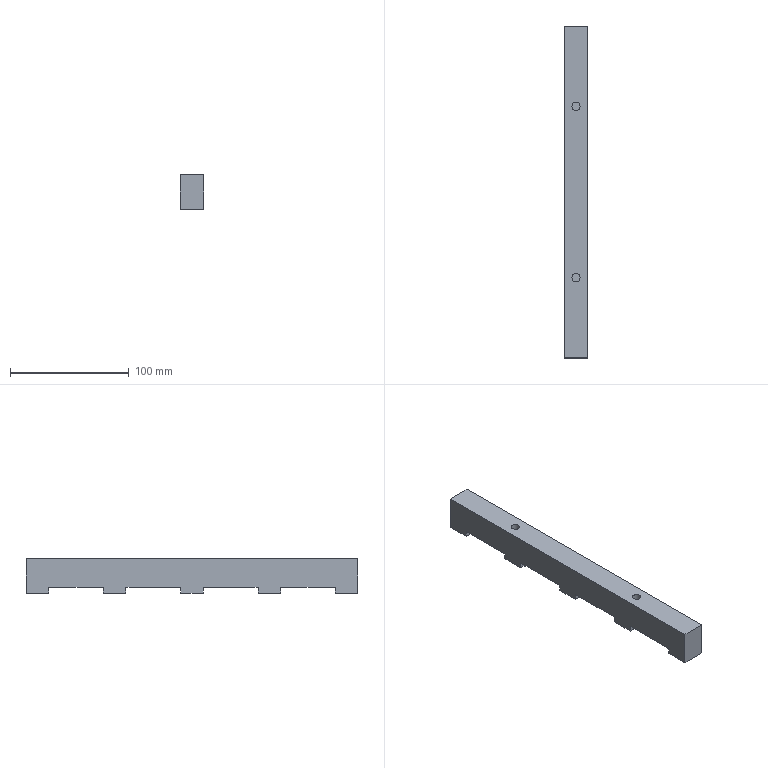Part | NX | 1 solid | 26 faces | box 20 x 279 x 29 mm | volume 142481 mm3 | plane 24 | cylinder 2 | commonest cylinder face diameters 6.88 x2
STEP:
#1=CARTESIAN_POINT('',(75.884,204.443,-119.05));
#2=VERTEX_POINT('',#1);
#3=CARTESIAN_POINT('',(72.444,204.443,-119.05));
#4=DIRECTION('',(0.,0.,-1.));
#5=DIRECTION('',(1.,0.,0.));
#6=AXIS2_PLACEMENT_3D('',#3,#4,#5);
#7=CIRCLE('',#6,3.44);
#8=EDGE_CURVE('',#2,#2,#7,.T.);
#9=ORIENTED_EDGE('',*,*,#8,.T.);
#10=EDGE_LOOP('',(#9));
#11=FACE_BOUND('',#10,.T.);
#12=CARTESIAN_POINT('',(75.884,204.443,-106.3));
#13=VERTEX_POINT('',#12);
#14=CARTESIAN_POINT('',(72.444,204.443,-106.3));
#15=DIRECTION('',(0.,0.,1.));
#16=DIRECTION('',(1.,0.,0.));
#17=AXIS2_PLACEMENT_3D('',#14,#15,#16);
#18=CIRCLE('',#17,3.44);
#19=EDGE_CURVE('',#13,#13,#18,.T.);
#20=ORIENTED_EDGE('',*,*,#19,.T.);
#21=EDGE_LOOP('',(#20));
#22=FACE_BOUND('',#21,.T.);
#23=CARTESIAN_POINT('',(72.444,204.443,-99.05));
#24=DIRECTION('',(0.,0.,-1.));
#25=DIRECTION('',(1.,0.,0.));
#26=AXIS2_PLACEMENT_3D('',#23,#24,#25);
#27=CYLINDRICAL_SURFACE('',#26,3.44);
#28=ADVANCED_FACE('',(#11,#22),#27,.F.);
#29=ORIENTED_EDGE('',*,*,#8,.F.);
#30=EDGE_LOOP('',(#29));
#31=FACE_BOUND('',#30,.T.);
#32=CARTESIAN_POINT('',(72.444,204.443,-119.05));
#33=DIRECTION('',(0.,0.,-1.));
#34=DIRECTION('',(-1.,0.,0.));
#35=AXIS2_PLACEMENT_3D('',#32,#33,#34);
#36=PLANE('',#35);
#37=ADVANCED_FACE('',(#31),#36,.F.);
#38=CARTESIAN_POINT('',(75.884,348.443,-118.8));
#39=VERTEX_POINT('',#38);
#40=CARTESIAN_POINT('',(72.444,348.443,-118.8));
#41=DIRECTION('',(0.,0.,-1.));
#42=DIRECTION('',(1.,0.,0.));
#43=AXIS2_PLACEMENT_3D('',#40,#41,#42);
#44=CIRCLE('',#43,3.44);
#45=EDGE_CURVE('',#39,#39,#44,.T.);
#46=ORIENTED_EDGE('',*,*,#45,.T.);
#47=EDGE_LOOP('',(#46));
#48=FACE_BOUND('',#47,.T.);
#49=CARTESIAN_POINT('',(75.884,348.443,-106.3));
#50=VERTEX_POINT('',#49);
#51=CARTESIAN_POINT('',(72.444,348.443,-106.3));
#52=DIRECTION('',(0.,0.,1.));
#53=DIRECTION('',(1.,0.,0.));
#54=AXIS2_PLACEMENT_3D('',#51,#52,#53);
#55=CIRCLE('',#54,3.44);
#56=EDGE_CURVE('',#50,#50,#55,.T.);
#57=ORIENTED_EDGE('',*,*,#56,.T.);
#58=EDGE_LOOP('',(#57));
#59=FACE_BOUND('',#58,.T.);
#60=CARTESIAN_POINT('',(72.444,348.443,-98.8));
#61=DIRECTION('',(0.,0.,-1.));
#62=DIRECTION('',(1.,0.,0.));
#63=AXIS2_PLACEMENT_3D('',#60,#61,#62);
#64=CYLINDRICAL_SURFACE('',#63,3.44);
#65=ADVANCED_FACE('',(#48,#59),#64,.F.);
#66=ORIENTED_EDGE('',*,*,#45,.F.);
#67=EDGE_LOOP('',(#66));
#68=FACE_BOUND('',#67,.T.);
#69=CARTESIAN_POINT('',(72.444,348.443,-118.8));
#70=DIRECTION('',(0.,0.,-1.));
#71=DIRECTION('',(-1.,0.,0.));
#72=AXIS2_PLACEMENT_3D('',#69,#70,#71);
#73=PLANE('',#72);
#74=ADVANCED_FACE('',(#68),#73,.F.);
#75=CARTESIAN_POINT('',(82.444,155.943,-130.3));
#76=VERTEX_POINT('',#75);
#77=CARTESIAN_POINT('',(82.444,155.943,-135.3));
#78=VERTEX_POINT('',#77);
#79=CARTESIAN_POINT('',(82.444,155.943,-130.75));
#80=DIRECTION('',(0.,0.,-1.));
#81=VECTOR('',#80,1000.);
#82=LINE('',#79,#81);
#83=EDGE_CURVE('',#76,#78,#82,.T.);
#84=ORIENTED_EDGE('',*,*,#83,.T.);
#85=CARTESIAN_POINT('',(62.444,155.943,-135.3));
#86=VERTEX_POINT('',#85);
#87=CARTESIAN_POINT('',(72.444,155.943,-135.3));
#88=DIRECTION('',(-1.,0.,0.));
#89=VECTOR('',#88,1000.);
#90=LINE('',#87,#89);
#91=EDGE_CURVE('',#78,#86,#90,.T.);
#92=ORIENTED_EDGE('',*,*,#91,.T.);
#93=CARTESIAN_POINT('',(62.444,155.943,-130.3));
#94=VERTEX_POINT('',#93);
#95=CARTESIAN_POINT('',(62.444,155.943,-139.8));
#96=DIRECTION('',(0.,0.,-1.));
#97=VECTOR('',#96,1000.);
#98=LINE('',#95,#97);
#99=EDGE_CURVE('',#94,#86,#98,.T.);
#100=ORIENTED_EDGE('',*,*,#99,.F.);
#101=CARTESIAN_POINT('',(113.544,155.943,-130.3));
#102=DIRECTION('',(1.,0.,0.));
#103=VECTOR('',#102,1000.);
#104=LINE('',#101,#103);
#105=EDGE_CURVE('',#94,#76,#104,.T.);
#106=ORIENTED_EDGE('',*,*,#105,.T.);
#107=EDGE_LOOP('',(#84,#92,#100,#106));
#108=FACE_BOUND('',#107,.T.);
#109=CARTESIAN_POINT('',(113.544,155.943,-130.75));
#110=DIRECTION('',(0.,1.,0.));
#111=DIRECTION('',(-1.,0.,0.));
#112=AXIS2_PLACEMENT_3D('',#109,#110,#111);
#113=PLANE('',#112);
#114=ADVANCED_FACE('',(#108),#113,.T.);
#115=CARTESIAN_POINT('',(62.444,201.943,-135.3));
#116=VERTEX_POINT('',#115);
#117=CARTESIAN_POINT('',(62.444,201.943,-130.3));
#118=VERTEX_POINT('',#117);
#119=CARTESIAN_POINT('',(62.444,201.943,-139.8));
#120=DIRECTION('',(0.,0.,1.));
#121=VECTOR('',#120,1000.);
#122=LINE('',#119,#121);
#123=EDGE_CURVE('',#116,#118,#122,.T.);
#124=ORIENTED_EDGE('',*,*,#123,.F.);
#125=CARTESIAN_POINT('',(82.444,201.943,-135.3));
#126=VERTEX_POINT('',#125);
#127=CARTESIAN_POINT('',(72.444,201.943,-135.3));
#128=DIRECTION('',(1.,0.,0.));
#129=VECTOR('',#128,1000.);
#130=LINE('',#127,#129);
#131=EDGE_CURVE('',#116,#126,#130,.T.);
#132=ORIENTED_EDGE('',*,*,#131,.T.);
#133=CARTESIAN_POINT('',(82.444,201.943,-130.3));
#134=VERTEX_POINT('',#133);
#135=CARTESIAN_POINT('',(82.444,201.943,-139.85));
#136=DIRECTION('',(0.,0.,1.));
#137=VECTOR('',#136,1000.);
#138=LINE('',#135,#137);
#139=EDGE_CURVE('',#126,#134,#138,.T.);
#140=ORIENTED_EDGE('',*,*,#139,.T.);
#141=CARTESIAN_POINT('',(72.444,201.943,-130.3));
#142=DIRECTION('',(-1.,0.,0.));
#143=VECTOR('',#142,1000.);
#144=LINE('',#141,#143);
#145=EDGE_CURVE('',#134,#118,#144,.T.);
#146=ORIENTED_EDGE('',*,*,#145,.T.);
#147=EDGE_LOOP('',(#124,#132,#140,#146));
#148=FACE_BOUND('',#147,.T.);
#149=CARTESIAN_POINT('',(113.544,201.943,-139.85));
#150=DIRECTION('',(0.,-1.,0.));
#151=DIRECTION('',(1.,0.,0.));
#152=AXIS2_PLACEMENT_3D('',#149,#150,#151);
#153=PLANE('',#152);
#154=ADVANCED_FACE('',(#148),#153,.T.);
#155=CARTESIAN_POINT('',(82.444,220.943,-130.3));
#156=VERTEX_POINT('',#155);
#157=CARTESIAN_POINT('',(82.444,220.943,-135.3));
#158=VERTEX_POINT('',#157);
#159=CARTESIAN_POINT('',(82.444,220.943,-130.75));
#160=DIRECTION('',(0.,0.,-1.));
#161=VECTOR('',#160,1000.);
#162=LINE('',#159,#161);
#163=EDGE_CURVE('',#156,#158,#162,.T.);
#164=ORIENTED_EDGE('',*,*,#163,.T.);
#165=CARTESIAN_POINT('',(62.444,220.943,-135.3));
#166=VERTEX_POINT('',#165);
#167=CARTESIAN_POINT('',(72.444,220.943,-135.3));
#168=DIRECTION('',(-1.,0.,0.));
#169=VECTOR('',#168,1000.);
#170=LINE('',#167,#169);
#171=EDGE_CURVE('',#158,#166,#170,.T.);
#172=ORIENTED_EDGE('',*,*,#171,.T.);
#173=CARTESIAN_POINT('',(62.444,220.943,-130.3));
#174=VERTEX_POINT('',#173);
#175=CARTESIAN_POINT('',(62.444,220.943,-139.8));
#176=DIRECTION('',(0.,0.,-1.));
#177=VECTOR('',#176,1000.);
#178=LINE('',#175,#177);
#179=EDGE_CURVE('',#174,#166,#178,.T.);
#180=ORIENTED_EDGE('',*,*,#179,.F.);
#181=CARTESIAN_POINT('',(113.544,220.943,-130.3));
#182=DIRECTION('',(1.,0.,0.));
#183=VECTOR('',#182,1000.);
#184=LINE('',#181,#183);
#185=EDGE_CURVE('',#174,#156,#184,.T.);
#186=ORIENTED_EDGE('',*,*,#185,.T.);
#187=EDGE_LOOP('',(#164,#172,#180,#186));
#188=FACE_BOUND('',#187,.T.);
#189=CARTESIAN_POINT('',(113.544,220.943,-130.75));
#190=DIRECTION('',(0.,1.,0.));
#191=DIRECTION('',(-1.,0.,0.));
#192=AXIS2_PLACEMENT_3D('',#189,#190,#191);
#193=PLANE('',#192);
#194=ADVANCED_FACE('',(#188),#193,.T.);
#195=CARTESIAN_POINT('',(62.444,266.943,-135.3));
#196=VERTEX_POINT('',#195);
#197=CARTESIAN_POINT('',(62.444,266.943,-130.3));
#198=VERTEX_POINT('',#197);
#199=CARTESIAN_POINT('',(62.444,266.943,-139.8));
#200=DIRECTION('',(0.,0.,1.));
#201=VECTOR('',#200,1000.);
#202=LINE('',#199,#201);
#203=EDGE_CURVE('',#196,#198,#202,.T.);
#204=ORIENTED_EDGE('',*,*,#203,.F.);
#205=CARTESIAN_POINT('',(82.444,266.943,-135.3));
#206=VERTEX_POINT('',#205);
#207=CARTESIAN_POINT('',(72.444,266.943,-135.3));
#208=DIRECTION('',(1.,0.,0.));
#209=VECTOR('',#208,1000.);
#210=LINE('',#207,#209);
#211=EDGE_CURVE('',#196,#206,#210,.T.);
#212=ORIENTED_EDGE('',*,*,#211,.T.);
#213=CARTESIAN_POINT('',(82.444,266.943,-130.3));
#214=VERTEX_POINT('',#213);
#215=CARTESIAN_POINT('',(82.444,266.943,-139.85));
#216=DIRECTION('',(0.,0.,1.));
#217=VECTOR('',#216,1000.);
#218=LINE('',#215,#217);
#219=EDGE_CURVE('',#206,#214,#218,.T.);
#220=ORIENTED_EDGE('',*,*,#219,.T.);
#221=CARTESIAN_POINT('',(113.544,266.943,-130.3));
#222=DIRECTION('',(-1.,0.,0.));
#223=VECTOR('',#222,1000.);
#224=LINE('',#221,#223);
#225=EDGE_CURVE('',#214,#198,#224,.T.);
#226=ORIENTED_EDGE('',*,*,#225,.T.);
#227=EDGE_LOOP('',(#204,#212,#220,#226));
#228=FACE_BOUND('',#227,.T.);
#229=CARTESIAN_POINT('',(113.544,266.943,-139.85));
#230=DIRECTION('',(0.,-1.,0.));
#231=DIRECTION('',(1.,0.,0.));
#232=AXIS2_PLACEMENT_3D('',#229,#230,#231);
#233=PLANE('',#232);
#234=ADVANCED_FACE('',(#228),#233,.T.);
#235=CARTESIAN_POINT('',(82.444,285.943,-130.3));
#236=VERTEX_POINT('',#235);
#237=CARTESIAN_POINT('',(82.444,285.943,-135.3));
#238=VERTEX_POINT('',#237);
#239=CARTESIAN_POINT('',(82.444,285.943,-130.75));
#240=DIRECTION('',(0.,0.,-1.));
#241=VECTOR('',#240,1000.);
#242=LINE('',#239,#241);
#243=EDGE_CURVE('',#236,#238,#242,.T.);
#244=ORIENTED_EDGE('',*,*,#243,.T.);
#245=CARTESIAN_POINT('',(62.444,285.943,-135.3));
#246=VERTEX_POINT('',#245);
#247=CARTESIAN_POINT('',(72.444,285.943,-135.3));
#248=DIRECTION('',(-1.,0.,0.));
#249=VECTOR('',#248,1000.);
#250=LINE('',#247,#249);
#251=EDGE_CURVE('',#238,#246,#250,.T.);
#252=ORIENTED_EDGE('',*,*,#251,.T.);
#253=CARTESIAN_POINT('',(62.444,285.943,-130.3));
#254=VERTEX_POINT('',#253);
#255=CARTESIAN_POINT('',(62.444,285.943,-139.8));
#256=DIRECTION('',(0.,0.,-1.));
#257=VECTOR('',#256,1000.);
#258=LINE('',#255,#257);
#259=EDGE_CURVE('',#254,#246,#258,.T.);
#260=ORIENTED_EDGE('',*,*,#259,.F.);
#261=CARTESIAN_POINT('',(113.544,285.943,-130.3));
#262=DIRECTION('',(1.,0.,0.));
#263=VECTOR('',#262,1000.);
#264=LINE('',#261,#263);
#265=EDGE_CURVE('',#254,#236,#264,.T.);
#266=ORIENTED_EDGE('',*,*,#265,.T.);
#267=EDGE_LOOP('',(#244,#252,#260,#266));
#268=FACE_BOUND('',#267,.T.);
#269=CARTESIAN_POINT('',(113.544,285.943,-130.75));
#270=DIRECTION('',(0.,1.,0.));
#271=DIRECTION('',(-1.,0.,0.));
#272=AXIS2_PLACEMENT_3D('',#269,#270,#271);
#273=PLANE('',#272);
#274=ADVANCED_FACE('',(#268),#273,.T.);
#275=CARTESIAN_POINT('',(62.444,331.943,-135.3));
#276=VERTEX_POINT('',#275);
#277=CARTESIAN_POINT('',(62.444,331.943,-130.3));
#278=VERTEX_POINT('',#277);
#279=CARTESIAN_POINT('',(62.444,331.943,-139.8));
#280=DIRECTION('',(0.,0.,1.));
#281=VECTOR('',#280,1000.);
#282=LINE('',#279,#281);
#283=EDGE_CURVE('',#276,#278,#282,.T.);
#284=ORIENTED_EDGE('',*,*,#283,.F.);
#285=CARTESIAN_POINT('',(82.444,331.943,-135.3));
#286=VERTEX_POINT('',#285);
#287=CARTESIAN_POINT('',(72.444,331.943,-135.3));
#288=DIRECTION('',(1.,0.,0.));
#289=VECTOR('',#288,1000.);
#290=LINE('',#287,#289);
#291=EDGE_CURVE('',#276,#286,#290,.T.);
#292=ORIENTED_EDGE('',*,*,#291,.T.);
#293=CARTESIAN_POINT('',(82.444,331.943,-130.3));
#294=VERTEX_POINT('',#293);
#295=CARTESIAN_POINT('',(82.444,331.943,-139.85));
#296=DIRECTION('',(0.,0.,1.));
#297=VECTOR('',#296,1000.);
#298=LINE('',#295,#297);
#299=EDGE_CURVE('',#286,#294,#298,.T.);
#300=ORIENTED_EDGE('',*,*,#299,.T.);
#301=CARTESIAN_POINT('',(113.544,331.943,-130.3));
#302=DIRECTION('',(-1.,0.,0.));
#303=VECTOR('',#302,1000.);
#304=LINE('',#301,#303);
#305=EDGE_CURVE('',#294,#278,#304,.T.);
#306=ORIENTED_EDGE('',*,*,#305,.T.);
#307=EDGE_LOOP('',(#284,#292,#300,#306));
#308=FACE_BOUND('',#307,.T.);
#309=CARTESIAN_POINT('',(113.544,331.943,-139.85));
#310=DIRECTION('',(0.,-1.,0.));
#311=DIRECTION('',(1.,0.,0.));
#312=AXIS2_PLACEMENT_3D('',#309,#310,#311);
#313=PLANE('',#312);
#314=ADVANCED_FACE('',(#308),#313,.T.);
#315=CARTESIAN_POINT('',(82.444,350.943,-130.3));
#316=VERTEX_POINT('',#315);
#317=CARTESIAN_POINT('',(82.444,350.943,-135.3));
#318=VERTEX_POINT('',#317);
#319=CARTESIAN_POINT('',(82.444,350.943,-130.75));
#320=DIRECTION('',(0.,0.,-1.));
#321=VECTOR('',#320,1000.);
#322=LINE('',#319,#321);
#323=EDGE_CURVE('',#316,#318,#322,.T.);
#324=ORIENTED_EDGE('',*,*,#323,.T.);
#325=CARTESIAN_POINT('',(62.444,350.943,-135.3));
#326=VERTEX_POINT('',#325);
#327=CARTESIAN_POINT('',(72.444,350.943,-135.3));
#328=DIRECTION('',(-1.,0.,0.));
#329=VECTOR('',#328,1000.);
#330=LINE('',#327,#329);
#331=EDGE_CURVE('',#318,#326,#330,.T.);
#332=ORIENTED_EDGE('',*,*,#331,.T.);
#333=CARTESIAN_POINT('',(62.444,350.943,-130.3));
#334=VERTEX_POINT('',#333);
#335=CARTESIAN_POINT('',(62.444,350.943,-139.8));
#336=DIRECTION('',(0.,0.,-1.));
#337=VECTOR('',#336,1000.);
#338=LINE('',#335,#337);
#339=EDGE_CURVE('',#334,#326,#338,.T.);
#340=ORIENTED_EDGE('',*,*,#339,.F.);
#341=CARTESIAN_POINT('',(113.544,350.943,-130.3));
#342=DIRECTION('',(1.,0.,0.));
#343=VECTOR('',#342,1000.);
#344=LINE('',#341,#343);
#345=EDGE_CURVE('',#334,#316,#344,.T.);
#346=ORIENTED_EDGE('',*,*,#345,.T.);
#347=EDGE_LOOP('',(#324,#332,#340,#346));
#348=FACE_BOUND('',#347,.T.);
#349=CARTESIAN_POINT('',(113.544,350.943,-130.75));
#350=DIRECTION('',(0.,1.,0.));
#351=DIRECTION('',(-1.,0.,0.));
#352=AXIS2_PLACEMENT_3D('',#349,#350,#351);
#353=PLANE('',#352);
#354=ADVANCED_FACE('',(#348),#353,.T.);
#355=CARTESIAN_POINT('',(62.444,396.943,-135.3));
#356=VERTEX_POINT('',#355);
#357=CARTESIAN_POINT('',(62.444,396.943,-130.3));
#358=VERTEX_POINT('',#357);
#359=CARTESIAN_POINT('',(62.444,396.943,-139.8));
#360=DIRECTION('',(0.,0.,1.));
#361=VECTOR('',#360,1000.);
#362=LINE('',#359,#361);
#363=EDGE_CURVE('',#356,#358,#362,.T.);
#364=ORIENTED_EDGE('',*,*,#363,.F.);
#365=CARTESIAN_POINT('',(82.444,396.943,-135.3));
#366=VERTEX_POINT('',#365);
#367=CARTESIAN_POINT('',(72.444,396.943,-135.3));
#368=DIRECTION('',(1.,0.,0.));
#369=VECTOR('',#368,1000.);
#370=LINE('',#367,#369);
#371=EDGE_CURVE('',#356,#366,#370,.T.);
#372=ORIENTED_EDGE('',*,*,#371,.T.);
#373=CARTESIAN_POINT('',(82.444,396.943,-130.3));
#374=VERTEX_POINT('',#373);
#375=CARTESIAN_POINT('',(82.444,396.943,-139.85));
#376=DIRECTION('',(0.,0.,1.));
#377=VECTOR('',#376,1000.);
#378=LINE('',#375,#377);
#379=EDGE_CURVE('',#366,#374,#378,.T.);
#380=ORIENTED_EDGE('',*,*,#379,.T.);
#381=CARTESIAN_POINT('',(113.544,396.943,-130.3));
#382=DIRECTION('',(-1.,0.,0.));
#383=VECTOR('',#382,1000.);
#384=LINE('',#381,#383);
#385=EDGE_CURVE('',#374,#358,#384,.T.);
#386=ORIENTED_EDGE('',*,*,#385,.T.);
#387=EDGE_LOOP('',(#364,#372,#380,#386));
#388=FACE_BOUND('',#387,.T.);
#389=CARTESIAN_POINT('',(113.544,396.943,-139.85));
#390=DIRECTION('',(0.,-1.,0.));
#391=DIRECTION('',(1.,0.,0.));
#392=AXIS2_PLACEMENT_3D('',#389,#390,#391);
#393=PLANE('',#392);
#394=ADVANCED_FACE('',(#388),#393,.T.);
#395=CARTESIAN_POINT('',(82.444,415.943,-106.3));
#396=VERTEX_POINT('',#395);
#397=CARTESIAN_POINT('',(82.444,415.943,-135.3));
#398=VERTEX_POINT('',#397);
#399=CARTESIAN_POINT('',(82.444,415.943,-134.85));
#400=DIRECTION('',(0.,0.,-1.));
#401=VECTOR('',#400,1000.);
#402=LINE('',#399,#401);
#403=EDGE_CURVE('',#396,#398,#402,.T.);
#404=ORIENTED_EDGE('',*,*,#403,.T.);
#405=CARTESIAN_POINT('',(62.444,415.943,-135.3));
#406=VERTEX_POINT('',#405);
#407=CARTESIAN_POINT('',(72.444,415.943,-135.3));
#408=DIRECTION('',(-1.,0.,0.));
#409=VECTOR('',#408,1000.);
#410=LINE('',#407,#409);
#411=EDGE_CURVE('',#398,#406,#410,.T.);
#412=ORIENTED_EDGE('',*,*,#411,.T.);
#413=CARTESIAN_POINT('',(62.444,415.943,-106.3));
#414=VERTEX_POINT('',#413);
#415=CARTESIAN_POINT('',(62.444,415.943,-139.8));
#416=DIRECTION('',(0.,0.,-1.));
#417=VECTOR('',#416,1000.);
#418=LINE('',#415,#417);
#419=EDGE_CURVE('',#414,#406,#418,.T.);
#420=ORIENTED_EDGE('',*,*,#419,.F.);
#421=CARTESIAN_POINT('',(181.344,415.943,-106.3));
#422=DIRECTION('',(-1.,0.,0.));
#423=VECTOR('',#422,1000.);
#424=LINE('',#421,#423);
#425=EDGE_CURVE('',#396,#414,#424,.T.);
#426=ORIENTED_EDGE('',*,*,#425,.F.);
#427=EDGE_LOOP('',(#404,#412,#420,#426));
#428=FACE_BOUND('',#427,.T.);
#429=CARTESIAN_POINT('',(113.544,415.943,-134.85));
#430=DIRECTION('',(0.,1.,0.));
#431=DIRECTION('',(-1.,0.,0.));
#432=AXIS2_PLACEMENT_3D('',#429,#430,#431);
#433=PLANE('',#432);
#434=ADVANCED_FACE('',(#428),#433,.T.);
#435=CARTESIAN_POINT('',(82.444,136.943,-106.3));
#436=VERTEX_POINT('',#435);
#437=CARTESIAN_POINT('',(82.444,-139.057,-106.3));
#438=DIRECTION('',(0.,1.,0.));
#439=VECTOR('',#438,1000.);
#440=LINE('',#437,#439);
#441=EDGE_CURVE('',#436,#396,#440,.T.);
#442=ORIENTED_EDGE('',*,*,#441,.F.);
#443=CARTESIAN_POINT('',(82.444,136.943,-135.3));
#444=VERTEX_POINT('',#443);
#445=CARTESIAN_POINT('',(82.444,136.943,-139.85));
#446=DIRECTION('',(0.,0.,1.));
#447=VECTOR('',#446,1000.);
#448=LINE('',#445,#447);
#449=EDGE_CURVE('',#444,#436,#448,.T.);
#450=ORIENTED_EDGE('',*,*,#449,.F.);
#451=CARTESIAN_POINT('',(82.444,-120.057,-135.3));
#452=DIRECTION('',(0.,1.,0.));
#453=VECTOR('',#452,1000.);
#454=LINE('',#451,#453);
#455=EDGE_CURVE('',#444,#78,#454,.T.);
#456=ORIENTED_EDGE('',*,*,#455,.T.);
#457=ORIENTED_EDGE('',*,*,#83,.F.);
#458=CARTESIAN_POINT('',(82.444,-132.757,-130.3));
#459=DIRECTION('',(0.,-1.,0.));
#460=VECTOR('',#459,1000.);
#461=LINE('',#458,#460);
#462=EDGE_CURVE('',#134,#76,#461,.T.);
#463=ORIENTED_EDGE('',*,*,#462,.F.);
#464=ORIENTED_EDGE('',*,*,#139,.F.);
#465=CARTESIAN_POINT('',(82.444,-134.057,-135.3));
#466=DIRECTION('',(0.,1.,0.));
#467=VECTOR('',#466,1000.);
#468=LINE('',#465,#467);
#469=EDGE_CURVE('',#126,#158,#468,.T.);
#470=ORIENTED_EDGE('',*,*,#469,.T.);
#471=ORIENTED_EDGE('',*,*,#163,.F.);
#472=CARTESIAN_POINT('',(82.444,-11.757,-130.3));
#473=DIRECTION('',(0.,-1.,0.));
#474=VECTOR('',#473,1000.);
#475=LINE('',#472,#474);
#476=EDGE_CURVE('',#214,#156,#475,.T.);
#477=ORIENTED_EDGE('',*,*,#476,.F.);
#478=ORIENTED_EDGE('',*,*,#219,.F.);
#479=CARTESIAN_POINT('',(82.444,-134.057,-135.3));
#480=DIRECTION('',(0.,1.,0.));
#481=VECTOR('',#480,1000.);
#482=LINE('',#479,#481);
#483=EDGE_CURVE('',#206,#238,#482,.T.);
#484=ORIENTED_EDGE('',*,*,#483,.T.);
#485=ORIENTED_EDGE('',*,*,#243,.F.);
#486=CARTESIAN_POINT('',(82.444,-11.757,-130.3));
#487=DIRECTION('',(0.,-1.,0.));
#488=VECTOR('',#487,1000.);
#489=LINE('',#486,#488);
#490=EDGE_CURVE('',#294,#236,#489,.T.);
#491=ORIENTED_EDGE('',*,*,#490,.F.);
#492=ORIENTED_EDGE('',*,*,#299,.F.);
#493=CARTESIAN_POINT('',(82.444,-134.057,-135.3));
#494=DIRECTION('',(0.,1.,0.));
#495=VECTOR('',#494,1000.);
#496=LINE('',#493,#495);
#497=EDGE_CURVE('',#286,#318,#496,.T.);
#498=ORIENTED_EDGE('',*,*,#497,.T.);
#499=ORIENTED_EDGE('',*,*,#323,.F.);
#500=CARTESIAN_POINT('',(82.444,-11.757,-130.3));
#501=DIRECTION('',(0.,-1.,0.));
#502=VECTOR('',#501,1000.);
#503=LINE('',#500,#502);
#504=EDGE_CURVE('',#374,#316,#503,.T.);
#505=ORIENTED_EDGE('',*,*,#504,.F.);
#506=ORIENTED_EDGE('',*,*,#379,.F.);
#507=CARTESIAN_POINT('',(82.444,-134.057,-135.3));
#508=DIRECTION('',(0.,1.,0.));
#509=VECTOR('',#508,1000.);
#510=LINE('',#507,#509);
#511=EDGE_CURVE('',#366,#398,#510,.T.);
#512=ORIENTED_EDGE('',*,*,#511,.T.);
#513=ORIENTED_EDGE('',*,*,#403,.F.);
#514=EDGE_LOOP('',(#442,#450,#456,#457,#463,#464,#470,#471,#477,#478,#484,#485,#491,#492,#498,#499,#505,#506,#512,#513));
#515=FACE_BOUND('',#514,.T.);
#516=CARTESIAN_POINT('',(82.444,-134.057,-134.97));
#517=DIRECTION('',(1.,0.,0.));
#518=DIRECTION('',(0.,-1.,0.));
#519=AXIS2_PLACEMENT_3D('',#516,#517,#518);
#520=PLANE('',#519);
#521=ADVANCED_FACE('',(#515),#520,.T.);
#522=ORIENTED_EDGE('',*,*,#363,.T.);
#523=CARTESIAN_POINT('',(62.444,331.043,-130.3));
#524=DIRECTION('',(0.,-1.,0.));
#525=VECTOR('',#524,1000.);
#526=LINE('',#523,#525);
#527=EDGE_CURVE('',#358,#334,#526,.T.);
#528=ORIENTED_EDGE('',*,*,#527,.T.);
#529=ORIENTED_EDGE('',*,*,#339,.T.);
#530=CARTESIAN_POINT('',(62.444,-58.807,-135.3));
#531=DIRECTION('',(0.,1.,0.));
#532=VECTOR('',#531,1000.);
#533=LINE('',#530,#532);
#534=EDGE_CURVE('',#276,#326,#533,.T.);
#535=ORIENTED_EDGE('',*,*,#534,.F.);
#536=ORIENTED_EDGE('',*,*,#283,.T.);
#537=CARTESIAN_POINT('',(62.444,331.043,-130.3));
#538=DIRECTION('',(0.,-1.,0.));
#539=VECTOR('',#538,1000.);
#540=LINE('',#537,#539);
#541=EDGE_CURVE('',#278,#254,#540,.T.);
#542=ORIENTED_EDGE('',*,*,#541,.T.);
#543=ORIENTED_EDGE('',*,*,#259,.T.);
#544=CARTESIAN_POINT('',(62.444,-58.807,-135.3));
#545=DIRECTION('',(0.,1.,0.));
#546=VECTOR('',#545,1000.);
#547=LINE('',#544,#546);
#548=EDGE_CURVE('',#196,#246,#547,.T.);
#549=ORIENTED_EDGE('',*,*,#548,.F.);
#550=ORIENTED_EDGE('',*,*,#203,.T.);
#551=CARTESIAN_POINT('',(62.444,331.043,-130.3));
#552=DIRECTION('',(0.,-1.,0.));
#553=VECTOR('',#552,1000.);
#554=LINE('',#551,#553);
#555=EDGE_CURVE('',#198,#174,#554,.T.);
#556=ORIENTED_EDGE('',*,*,#555,.T.);
#557=ORIENTED_EDGE('',*,*,#179,.T.);
#558=CARTESIAN_POINT('',(62.444,-58.807,-135.3));
#559=DIRECTION('',(0.,1.,0.));
#560=VECTOR('',#559,1000.);
#561=LINE('',#558,#560);
#562=EDGE_CURVE('',#116,#166,#561,.T.);
#563=ORIENTED_EDGE('',*,*,#562,.F.);
#564=ORIENTED_EDGE('',*,*,#123,.T.);
#565=CARTESIAN_POINT('',(62.444,332.343,-130.3));
#566=DIRECTION('',(0.,-1.,0.));
#567=VECTOR('',#566,1000.);
#568=LINE('',#565,#567);
#569=EDGE_CURVE('',#118,#94,#568,.T.);
#570=ORIENTED_EDGE('',*,*,#569,.T.);
#571=ORIENTED_EDGE('',*,*,#99,.T.);
#572=CARTESIAN_POINT('',(62.444,136.943,-135.3));
#573=VERTEX_POINT('',#572);
#574=CARTESIAN_POINT('',(62.444,145.193,-135.3));
#575=DIRECTION('',(0.,1.,0.));
#576=VECTOR('',#575,1000.);
#577=LINE('',#574,#576);
#578=EDGE_CURVE('',#573,#86,#577,.T.);
#579=ORIENTED_EDGE('',*,*,#578,.F.);
#580=CARTESIAN_POINT('',(62.444,136.943,-106.3));
#581=VERTEX_POINT('',#580);
#582=CARTESIAN_POINT('',(62.444,136.943,-139.8));
#583=DIRECTION('',(0.,0.,1.));
#584=VECTOR('',#583,1000.);
#585=LINE('',#582,#584);
#586=EDGE_CURVE('',#573,#581,#585,.T.);
#587=ORIENTED_EDGE('',*,*,#586,.T.);
#588=CARTESIAN_POINT('',(62.444,331.043,-106.3));
#589=DIRECTION('',(0.,1.,0.));
#590=VECTOR('',#589,1000.);
#591=LINE('',#588,#590);
#592=EDGE_CURVE('',#581,#414,#591,.T.);
#593=ORIENTED_EDGE('',*,*,#592,.T.);
#594=ORIENTED_EDGE('',*,*,#419,.T.);
#595=CARTESIAN_POINT('',(62.444,-58.807,-135.3));
#596=DIRECTION('',(0.,1.,0.));
#597=VECTOR('',#596,1000.);
#598=LINE('',#595,#597);
#599=EDGE_CURVE('',#356,#406,#598,.T.);
#600=ORIENTED_EDGE('',*,*,#599,.F.);
#601=EDGE_LOOP('',(#522,#528,#529,#535,#536,#542,#543,#549,#550,#556,#557,#563,#564,#570,#571,#579,#587,#593,#594,#600));
#602=FACE_BOUND('',#601,.T.);
#603=CARTESIAN_POINT('',(62.444,331.043,-139.8));
#604=DIRECTION('',(1.,0.,0.));
#605=DIRECTION('',(0.,1.,0.));
#606=AXIS2_PLACEMENT_3D('',#603,#604,#605);
#607=PLANE('',#606);
#608=ADVANCED_FACE('',(#602),#607,.F.);
#609=ORIENTED_EDGE('',*,*,#586,.F.);
#610=CARTESIAN_POINT('',(72.444,136.943,-135.3));
#611=DIRECTION('',(1.,0.,0.));
#612=VECTOR('',#611,1000.);
#613=LINE('',#610,#612);
#614=EDGE_CURVE('',#573,#444,#613,.T.);
#615=ORIENTED_EDGE('',*,*,#614,.T.);
#616=ORIENTED_EDGE('',*,*,#449,.T.);
#617=CARTESIAN_POINT('',(181.344,136.943,-106.3));
#618=DIRECTION('',(1.,0.,0.));
#619=VECTOR('',#618,1000.);
#620=LINE('',#617,#619);
#621=EDGE_CURVE('',#581,#436,#620,.T.);
#622=ORIENTED_EDGE('',*,*,#621,.F.);
#623=EDGE_LOOP('',(#609,#615,#616,#622));
#624=FACE_BOUND('',#623,.T.);
#625=CARTESIAN_POINT('',(113.544,136.943,-139.85));
#626=DIRECTION('',(0.,-1.,0.));
#627=DIRECTION('',(1.,0.,0.));
#628=AXIS2_PLACEMENT_3D('',#625,#626,#627);
#629=PLANE('',#628);
#630=ADVANCED_FACE('',(#624),#629,.T.);
#631=ORIENTED_EDGE('',*,*,#425,.T.);
#632=ORIENTED_EDGE('',*,*,#592,.F.);
#633=ORIENTED_EDGE('',*,*,#621,.T.);
#634=ORIENTED_EDGE('',*,*,#441,.T.);
#635=EDGE_LOOP('',(#631,#632,#633,#634));
#636=FACE_BOUND('',#635,.T.);
#637=ORIENTED_EDGE('',*,*,#56,.F.);
#638=EDGE_LOOP('',(#637));
#639=FACE_BOUND('',#638,.T.);
#640=ORIENTED_EDGE('',*,*,#19,.F.);
#641=EDGE_LOOP('',(#640));
#642=FACE_BOUND('',#641,.T.);
#643=CARTESIAN_POINT('',(181.344,-139.057,-106.3));
#644=DIRECTION('',(0.,0.,1.));
#645=DIRECTION('',(1.,0.,0.));
#646=AXIS2_PLACEMENT_3D('',#643,#644,#645);
#647=PLANE('',#646);
#648=ADVANCED_FACE('',(#636,#639,#642),#647,.T.);
#649=ORIENTED_EDGE('',*,*,#105,.F.);
#650=ORIENTED_EDGE('',*,*,#569,.F.);
#651=ORIENTED_EDGE('',*,*,#145,.F.);
#652=ORIENTED_EDGE('',*,*,#462,.T.);
#653=EDGE_LOOP('',(#649,#650,#651,#652));
#654=FACE_BOUND('',#653,.T.);
#655=CARTESIAN_POINT('',(72.444,-11.757,-130.3));
#656=DIRECTION('',(0.,0.,-1.));
#657=DIRECTION('',(-1.,0.,0.));
#658=AXIS2_PLACEMENT_3D('',#655,#656,#657);
#659=PLANE('',#658);
#660=ADVANCED_FACE('',(#654),#659,.T.);
#661=ORIENTED_EDGE('',*,*,#345,.F.);
#662=ORIENTED_EDGE('',*,*,#527,.F.);
#663=ORIENTED_EDGE('',*,*,#385,.F.);
#664=ORIENTED_EDGE('',*,*,#504,.T.);
#665=EDGE_LOOP('',(#661,#662,#663,#664));
#666=FACE_BOUND('',#665,.T.);
#667=CARTESIAN_POINT('',(72.444,-11.757,-130.3));
#668=DIRECTION('',(0.,0.,-1.));
#669=DIRECTION('',(-1.,0.,0.));
#670=AXIS2_PLACEMENT_3D('',#667,#668,#669);
#671=PLANE('',#670);
#672=ADVANCED_FACE('',(#666),#671,.T.);
#673=ORIENTED_EDGE('',*,*,#265,.F.);
#674=ORIENTED_EDGE('',*,*,#541,.F.);
#675=ORIENTED_EDGE('',*,*,#305,.F.);
#676=ORIENTED_EDGE('',*,*,#490,.T.);
#677=EDGE_LOOP('',(#673,#674,#675,#676));
#678=FACE_BOUND('',#677,.T.);
#679=CARTESIAN_POINT('',(72.444,-11.757,-130.3));
#680=DIRECTION('',(0.,0.,-1.));
#681=DIRECTION('',(-1.,0.,0.));
#682=AXIS2_PLACEMENT_3D('',#679,#680,#681);
#683=PLANE('',#682);
#684=ADVANCED_FACE('',(#678),#683,.T.);
#685=ORIENTED_EDGE('',*,*,#185,.F.);
#686=ORIENTED_EDGE('',*,*,#555,.F.);
#687=ORIENTED_EDGE('',*,*,#225,.F.);
#688=ORIENTED_EDGE('',*,*,#476,.T.);
#689=EDGE_LOOP('',(#685,#686,#687,#688));
#690=FACE_BOUND('',#689,.T.);
#691=CARTESIAN_POINT('',(72.444,-11.757,-130.3));
#692=DIRECTION('',(0.,0.,-1.));
#693=DIRECTION('',(-1.,0.,0.));
#694=AXIS2_PLACEMENT_3D('',#691,#692,#693);
#695=PLANE('',#694);
#696=ADVANCED_FACE('',(#690),#695,.T.);
#697=ORIENTED_EDGE('',*,*,#455,.F.);
#698=ORIENTED_EDGE('',*,*,#614,.F.);
#699=ORIENTED_EDGE('',*,*,#578,.T.);
#700=ORIENTED_EDGE('',*,*,#91,.F.);
#701=EDGE_LOOP('',(#697,#698,#699,#700));
#702=FACE_BOUND('',#701,.T.);
#703=CARTESIAN_POINT('',(72.444,146.443,-135.3));
#704=DIRECTION('',(0.,0.,-1.));
#705=DIRECTION('',(-1.,0.,0.));
#706=AXIS2_PLACEMENT_3D('',#703,#704,#705);
#707=PLANE('',#706);
#708=ADVANCED_FACE('',(#702),#707,.T.);
#709=ORIENTED_EDGE('',*,*,#511,.F.);
#710=ORIENTED_EDGE('',*,*,#371,.F.);
#711=ORIENTED_EDGE('',*,*,#599,.T.);
#712=ORIENTED_EDGE('',*,*,#411,.F.);
#713=EDGE_LOOP('',(#709,#710,#711,#712));
#714=FACE_BOUND('',#713,.T.);
#715=CARTESIAN_POINT('',(72.444,406.443,-135.3));
#716=DIRECTION('',(0.,0.,-1.));
#717=DIRECTION('',(-1.,0.,0.));
#718=AXIS2_PLACEMENT_3D('',#715,#716,#717);
#719=PLANE('',#718);
#720=ADVANCED_FACE('',(#714),#719,.T.);
#721=ORIENTED_EDGE('',*,*,#497,.F.);
#722=ORIENTED_EDGE('',*,*,#291,.F.);
#723=ORIENTED_EDGE('',*,*,#534,.T.);
#724=ORIENTED_EDGE('',*,*,#331,.F.);
#725=EDGE_LOOP('',(#721,#722,#723,#724));
#726=FACE_BOUND('',#725,.T.);
#727=CARTESIAN_POINT('',(72.444,341.443,-135.3));
#728=DIRECTION('',(0.,0.,-1.));
#729=DIRECTION('',(-1.,0.,0.));
#730=AXIS2_PLACEMENT_3D('',#727,#728,#729);
#731=PLANE('',#730);
#732=ADVANCED_FACE('',(#726),#731,.T.);
#733=ORIENTED_EDGE('',*,*,#483,.F.);
#734=ORIENTED_EDGE('',*,*,#211,.F.);
#735=ORIENTED_EDGE('',*,*,#548,.T.);
#736=ORIENTED_EDGE('',*,*,#251,.F.);
#737=EDGE_LOOP('',(#733,#734,#735,#736));
#738=FACE_BOUND('',#737,.T.);
#739=CARTESIAN_POINT('',(72.444,276.443,-135.3));
#740=DIRECTION('',(0.,0.,-1.));
#741=DIRECTION('',(-1.,0.,0.));
#742=AXIS2_PLACEMENT_3D('',#739,#740,#741);
#743=PLANE('',#742);
#744=ADVANCED_FACE('',(#738),#743,.T.);
#745=ORIENTED_EDGE('',*,*,#469,.F.);
#746=ORIENTED_EDGE('',*,*,#131,.F.);
#747=ORIENTED_EDGE('',*,*,#562,.T.);
#748=ORIENTED_EDGE('',*,*,#171,.F.);
#749=EDGE_LOOP('',(#745,#746,#747,#748));
#750=FACE_BOUND('',#749,.T.);
#751=CARTESIAN_POINT('',(72.444,211.443,-135.3));
#752=DIRECTION('',(0.,0.,-1.));
#753=DIRECTION('',(-1.,0.,0.));
#754=AXIS2_PLACEMENT_3D('',#751,#752,#753);
#755=PLANE('',#754);
#756=ADVANCED_FACE('',(#750),#755,.T.);
#757=CLOSED_SHELL('',(#28,#37,#65,#74,#114,#154,#194,#234,#274,#314,#354,#394,#434,#521,#608,#630,#648,#660,#672,#684,#696,#708,#720,#732,#744,#756));
#758=MANIFOLD_SOLID_BREP('',#757);
#759=(LENGTH_UNIT()NAMED_UNIT(*)SI_UNIT(.MILLI.,.METRE.));
#760=UNCERTAINTY_MEASURE_WITH_UNIT(LENGTH_MEASURE(0.00001),#759,'','');
#761=(NAMED_UNIT(*)PLANE_ANGLE_UNIT()SI_UNIT($,.RADIAN.));
#762=(NAMED_UNIT(*)SI_UNIT($,.STERADIAN.)SOLID_ANGLE_UNIT());
#763=(GEOMETRIC_REPRESENTATION_CONTEXT(3)GLOBAL_UNCERTAINTY_ASSIGNED_CONTEXT((#760))GLOBAL_UNIT_ASSIGNED_CONTEXT((#759,#761,#762))REPRESENTATION_CONTEXT('',''));
#764=ADVANCED_BREP_SHAPE_REPRESENTATION('',(#758),#763);